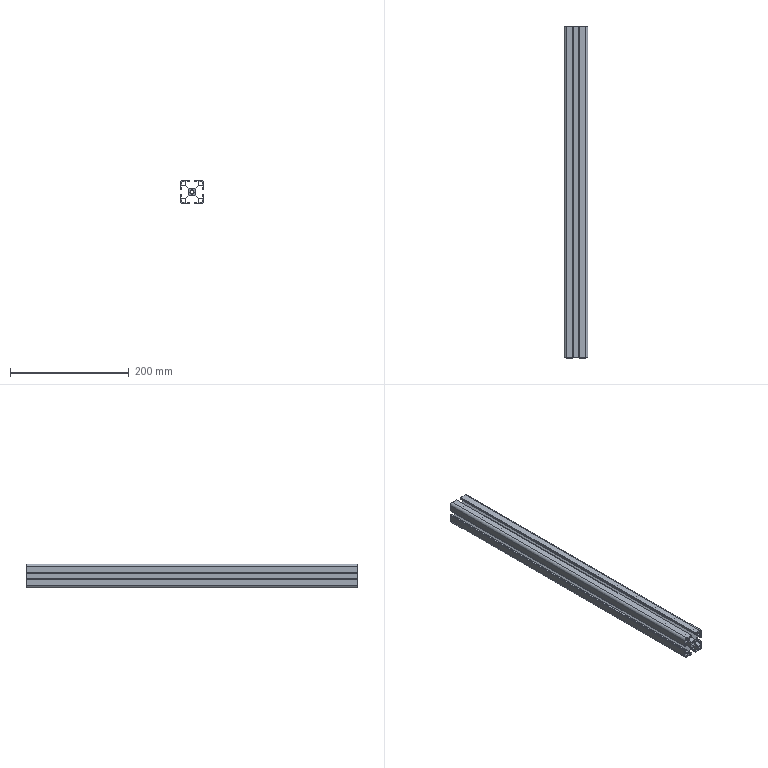Part | SolidWorks | features BaseBody 1 | 1 solid | 104 faces | box 40 x 560 x 40 mm | volume 265925 mm3 | plane 94 | cylinder 10 | commonest cylinder face diameters 5 x4 9 x4 6.8 x2